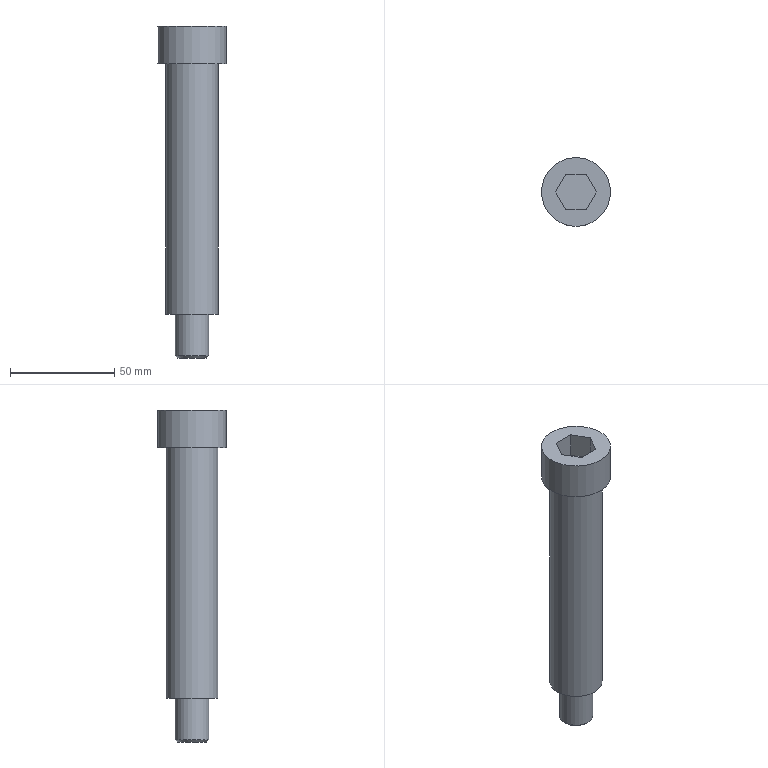Part | STEP file | solid 91 | 1 solid | 15 faces | box 33 x 33 x 159 mm | volume 75495 mm3 | plane 11 | cylinder 3 | cone 1 | commonest cylinder face diameters 16 x1 25 x1 33 x1